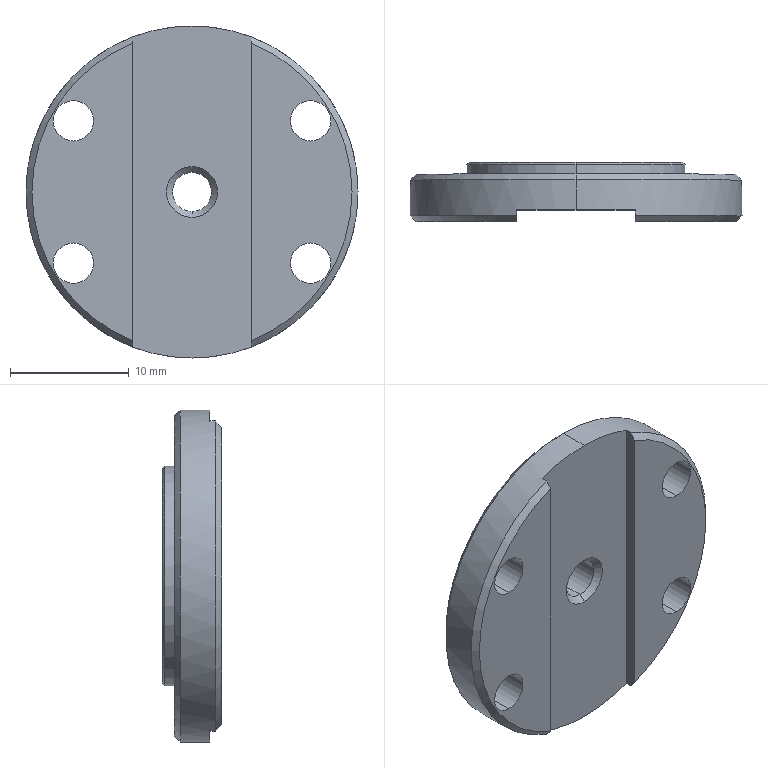Part | SolidWorks | features Chamfer 2, HoleWzd 2, ICE 2, Revolution 1 | 1 solid | 31 faces | box 28 x 5 x 28 mm | volume 2255 mm3 | cylinder 14 | cone 10 | plane 7 | commonest cylinder face diameters 3.4 x8 3.3 x2 18.5 x2 28 x2
STEP:
#1=CARTESIAN_POINT('',(0.,5.,9.05));
#2=VERTEX_POINT('',#1);
#3=CARTESIAN_POINT('',(0.,5.,-9.05));
#4=VERTEX_POINT('',#3);
#5=CARTESIAN_POINT('',(0.,5.,0.));
#6=DIRECTION('',(0.,1.,0.));
#7=DIRECTION('',(0.,0.,1.));
#8=AXIS2_PLACEMENT_3D('',#5,#6,#7);
#9=CIRCLE('',#8,9.05);
#10=EDGE_CURVE('',#2,#4,#9,.T.);
#11=ORIENTED_EDGE('',*,*,#10,.F.);
#12=CARTESIAN_POINT('',(0.,4.8,9.25));
#13=VERTEX_POINT('',#12);
#14=CARTESIAN_POINT('',(0.,5.,9.05));
#15=DIRECTION('',(0.,-0.7071,0.7071));
#16=VECTOR('',#15,1000.);
#17=LINE('',#14,#16);
#18=EDGE_CURVE('',#2,#13,#17,.T.);
#19=ORIENTED_EDGE('',*,*,#18,.T.);
#20=CARTESIAN_POINT('',(0.,4.8,-9.25));
#21=VERTEX_POINT('',#20);
#22=CARTESIAN_POINT('',(0.,4.8,0.));
#23=DIRECTION('',(0.,-1.,0.));
#24=DIRECTION('',(0.,0.,1.));
#25=AXIS2_PLACEMENT_3D('',#22,#23,#24);
#26=CIRCLE('',#25,9.25);
#27=EDGE_CURVE('',#21,#13,#26,.T.);
#28=ORIENTED_EDGE('',*,*,#27,.F.);
#29=CARTESIAN_POINT('',(0.,5.,-9.05));
#30=DIRECTION('',(0.,-0.7071,-0.7071));
#31=VECTOR('',#30,1000.);
#32=LINE('',#29,#31);
#33=EDGE_CURVE('',#4,#21,#32,.T.);
#34=ORIENTED_EDGE('',*,*,#33,.F.);
#35=EDGE_LOOP('',(#11,#19,#28,#34));
#36=FACE_OUTER_BOUND('',#35,.T.);
#37=CARTESIAN_POINT('',(0.,5.,0.));
#38=DIRECTION('',(0.,-1.,0.));
#39=DIRECTION('',(0.,0.,-1.));
#40=AXIS2_PLACEMENT_3D('',#37,#38,#39);
#41=CONICAL_SURFACE('',#40,9.05,0.7854);
#42=ADVANCED_FACE('',(#36),#41,.T.);
#43=CARTESIAN_POINT('',(0.,4.,13.5));
#44=VERTEX_POINT('',#43);
#45=CARTESIAN_POINT('',(0.,4.,-13.5));
#46=VERTEX_POINT('',#45);
#47=CARTESIAN_POINT('',(0.,4.,0.));
#48=DIRECTION('',(0.,1.,0.));
#49=DIRECTION('',(0.,0.,1.));
#50=AXIS2_PLACEMENT_3D('',#47,#48,#49);
#51=CIRCLE('',#50,13.5);
#52=EDGE_CURVE('',#44,#46,#51,.T.);
#53=ORIENTED_EDGE('',*,*,#52,.F.);
#54=CARTESIAN_POINT('',(0.,3.5,14.));
#55=VERTEX_POINT('',#54);
#56=CARTESIAN_POINT('',(0.,3.5,14.));
#57=DIRECTION('',(0.,-0.7071,0.7071));
#58=VECTOR('',#57,1000.);
#59=LINE('',#56,#58);
#60=EDGE_CURVE('',#44,#55,#59,.T.);
#61=ORIENTED_EDGE('',*,*,#60,.T.);
#62=CARTESIAN_POINT('',(0.,3.5,-14.));
#63=VERTEX_POINT('',#62);
#64=CARTESIAN_POINT('',(0.,3.5,0.));
#65=DIRECTION('',(0.,-1.,0.));
#66=DIRECTION('',(0.,0.,1.));
#67=AXIS2_PLACEMENT_3D('',#64,#65,#66);
#68=CIRCLE('',#67,14.);
#69=EDGE_CURVE('',#63,#55,#68,.T.);
#70=ORIENTED_EDGE('',*,*,#69,.F.);
#71=CARTESIAN_POINT('',(0.,3.5,-14.));
#72=DIRECTION('',(0.,-0.7071,-0.7071));
#73=VECTOR('',#72,1000.);
#74=LINE('',#71,#73);
#75=EDGE_CURVE('',#46,#63,#74,.T.);
#76=ORIENTED_EDGE('',*,*,#75,.F.);
#77=EDGE_LOOP('',(#53,#61,#70,#76));
#78=FACE_OUTER_BOUND('',#77,.T.);
#79=CARTESIAN_POINT('',(0.,3.5,0.));
#80=DIRECTION('',(0.,-1.,0.));
#81=DIRECTION('',(0.,0.,-1.));
#82=AXIS2_PLACEMENT_3D('',#79,#80,#81);
#83=CONICAL_SURFACE('',#82,14.,0.7854);
#84=ADVANCED_FACE('',(#78),#83,.T.);
#85=CARTESIAN_POINT('',(0.,4.5,-1.65));
#86=VERTEX_POINT('',#85);
#87=CARTESIAN_POINT('',(0.,4.5,1.65));
#88=VERTEX_POINT('',#87);
#89=CARTESIAN_POINT('',(0.,4.5,0.));
#90=DIRECTION('',(0.,1.,0.));
#91=DIRECTION('',(0.,0.,1.));
#92=AXIS2_PLACEMENT_3D('',#89,#90,#91);
#93=CIRCLE('',#92,1.65);
#94=EDGE_CURVE('',#86,#88,#93,.T.);
#95=ORIENTED_EDGE('',*,*,#94,.F.);
#96=CARTESIAN_POINT('',(0.,5.,-2.15));
#97=VERTEX_POINT('',#96);
#98=CARTESIAN_POINT('',(0.,4.5,-1.65));
#99=DIRECTION('',(0.,0.7071,-0.7071));
#100=VECTOR('',#99,1000.);
#101=LINE('',#98,#100);
#102=EDGE_CURVE('',#86,#97,#101,.T.);
#103=ORIENTED_EDGE('',*,*,#102,.T.);
#104=CARTESIAN_POINT('',(0.,5.,2.15));
#105=VERTEX_POINT('',#104);
#106=CARTESIAN_POINT('',(0.,5.,0.));
#107=DIRECTION('',(0.,-1.,0.));
#108=DIRECTION('',(0.,0.,1.));
#109=AXIS2_PLACEMENT_3D('',#106,#107,#108);
#110=CIRCLE('',#109,2.15);
#111=EDGE_CURVE('',#105,#97,#110,.T.);
#112=ORIENTED_EDGE('',*,*,#111,.F.);
#113=CARTESIAN_POINT('',(0.,4.5,1.65));
#114=DIRECTION('',(0.,0.7071,0.7071));
#115=VECTOR('',#114,1000.);
#116=LINE('',#113,#115);
#117=EDGE_CURVE('',#88,#105,#116,.T.);
#118=ORIENTED_EDGE('',*,*,#117,.F.);
#119=EDGE_LOOP('',(#95,#103,#112,#118));
#120=FACE_OUTER_BOUND('',#119,.T.);
#121=CARTESIAN_POINT('',(0.,4.5,0.));
#122=DIRECTION('',(0.,1.,0.));
#123=DIRECTION('',(0.,0.,1.));
#124=AXIS2_PLACEMENT_3D('',#121,#122,#123);
#125=CONICAL_SURFACE('',#124,1.65,0.7854);
#126=ADVANCED_FACE('',(#120),#125,.F.);
#127=CARTESIAN_POINT('',(0.,1.5,1.65));
#128=VERTEX_POINT('',#127);
#129=CARTESIAN_POINT('',(0.,1.5,-1.65));
#130=VERTEX_POINT('',#129);
#131=CARTESIAN_POINT('',(0.,1.5,0.));
#132=DIRECTION('',(0.,-1.,0.));
#133=DIRECTION('',(0.,0.,1.));
#134=AXIS2_PLACEMENT_3D('',#131,#132,#133);
#135=CIRCLE('',#134,1.65);
#136=EDGE_CURVE('',#128,#130,#135,.T.);
#137=ORIENTED_EDGE('',*,*,#136,.F.);
#138=CARTESIAN_POINT('',(0.,1.,2.15));
#139=VERTEX_POINT('',#138);
#140=CARTESIAN_POINT('',(0.,1.5,1.65));
#141=DIRECTION('',(0.,-0.7071,0.7071));
#142=VECTOR('',#141,1000.);
#143=LINE('',#140,#142);
#144=EDGE_CURVE('',#128,#139,#143,.T.);
#145=ORIENTED_EDGE('',*,*,#144,.T.);
#146=CARTESIAN_POINT('',(0.,1.,-2.15));
#147=VERTEX_POINT('',#146);
#148=CARTESIAN_POINT('',(0.,1.,0.));
#149=DIRECTION('',(0.,1.,0.));
#150=DIRECTION('',(0.,0.,1.));
#151=AXIS2_PLACEMENT_3D('',#148,#149,#150);
#152=CIRCLE('',#151,2.15);
#153=EDGE_CURVE('',#147,#139,#152,.T.);
#154=ORIENTED_EDGE('',*,*,#153,.F.);
#155=CARTESIAN_POINT('',(0.,1.5,-1.65));
#156=DIRECTION('',(0.,-0.7071,-0.7071));
#157=VECTOR('',#156,1000.);
#158=LINE('',#155,#157);
#159=EDGE_CURVE('',#130,#147,#158,.T.);
#160=ORIENTED_EDGE('',*,*,#159,.F.);
#161=EDGE_LOOP('',(#137,#145,#154,#160));
#162=FACE_OUTER_BOUND('',#161,.T.);
#163=CARTESIAN_POINT('',(0.,1.5,0.));
#164=DIRECTION('',(0.,-1.,0.));
#165=DIRECTION('',(0.,0.,-1.));
#166=AXIS2_PLACEMENT_3D('',#163,#164,#165);
#167=CONICAL_SURFACE('',#166,1.65,0.7854);
#168=ADVANCED_FACE('',(#162),#167,.F.);
#169=ORIENTED_EDGE('',*,*,#94,.T.);
#170=CARTESIAN_POINT('',(0.,1.,1.65));
#171=DIRECTION('',(0.,-1.,0.));
#172=VECTOR('',#171,1000.);
#173=LINE('',#170,#172);
#174=EDGE_CURVE('',#88,#128,#173,.T.);
#175=ORIENTED_EDGE('',*,*,#174,.T.);
#176=ORIENTED_EDGE('',*,*,#136,.T.);
#177=CARTESIAN_POINT('',(0.,1.,-1.65));
#178=DIRECTION('',(0.,-1.,0.));
#179=VECTOR('',#178,1000.);
#180=LINE('',#177,#179);
#181=EDGE_CURVE('',#86,#130,#180,.T.);
#182=ORIENTED_EDGE('',*,*,#181,.F.);
#183=EDGE_LOOP('',(#169,#175,#176,#182));
#184=FACE_OUTER_BOUND('',#183,.T.);
#185=CARTESIAN_POINT('',(0.,1.,0.));
#186=DIRECTION('',(0.,-1.,0.));
#187=DIRECTION('',(0.,0.,-1.));
#188=AXIS2_PLACEMENT_3D('',#185,#186,#187);
#189=CYLINDRICAL_SURFACE('',#188,1.65);
#190=ADVANCED_FACE('',(#184),#189,.F.);
#191=CARTESIAN_POINT('',(-10.,4.,4.3));
#192=VERTEX_POINT('',#191);
#193=CARTESIAN_POINT('',(-10.,4.,7.7));
#194=VERTEX_POINT('',#193);
#195=CARTESIAN_POINT('',(-10.,4.,6.));
#196=DIRECTION('',(0.,1.,0.));
#197=DIRECTION('',(0.,0.,1.));
#198=AXIS2_PLACEMENT_3D('',#195,#196,#197);
#199=CIRCLE('',#198,1.7);
#200=EDGE_CURVE('',#192,#194,#199,.T.);
#201=ORIENTED_EDGE('',*,*,#200,.T.);
#202=CARTESIAN_POINT('',(-10.,0.,7.7));
#203=VERTEX_POINT('',#202);
#204=CARTESIAN_POINT('',(-10.,0.,7.7));
#205=DIRECTION('',(0.,-1.,0.));
#206=VECTOR('',#205,1000.);
#207=LINE('',#204,#206);
#208=EDGE_CURVE('',#194,#203,#207,.T.);
#209=ORIENTED_EDGE('',*,*,#208,.T.);
#210=CARTESIAN_POINT('',(-10.,0.,4.3));
#211=VERTEX_POINT('',#210);
#212=CARTESIAN_POINT('',(-10.,0.,6.));
#213=DIRECTION('',(0.,-1.,0.));
#214=DIRECTION('',(0.,0.,-1.));
#215=AXIS2_PLACEMENT_3D('',#212,#213,#214);
#216=CIRCLE('',#215,1.7);
#217=EDGE_CURVE('',#203,#211,#216,.T.);
#218=ORIENTED_EDGE('',*,*,#217,.T.);
#219=CARTESIAN_POINT('',(-10.,0.,4.3));
#220=DIRECTION('',(0.,-1.,0.));
#221=VECTOR('',#220,1000.);
#222=LINE('',#219,#221);
#223=EDGE_CURVE('',#192,#211,#222,.T.);
#224=ORIENTED_EDGE('',*,*,#223,.F.);
#225=EDGE_LOOP('',(#201,#209,#218,#224));
#226=FACE_OUTER_BOUND('',#225,.T.);
#227=CARTESIAN_POINT('',(-10.,0.,6.));
#228=DIRECTION('',(0.,-1.,0.));
#229=DIRECTION('',(0.,0.,-1.));
#230=AXIS2_PLACEMENT_3D('',#227,#228,#229);
#231=CYLINDRICAL_SURFACE('',#230,1.7);
#232=ADVANCED_FACE('',(#226),#231,.F.);
#233=CARTESIAN_POINT('',(-10.,4.,-7.7));
#234=VERTEX_POINT('',#233);
#235=CARTESIAN_POINT('',(-10.,4.,-4.3));
#236=VERTEX_POINT('',#235);
#237=CARTESIAN_POINT('',(-10.,4.,-6.));
#238=DIRECTION('',(0.,1.,0.));
#239=DIRECTION('',(0.,0.,1.));
#240=AXIS2_PLACEMENT_3D('',#237,#238,#239);
#241=CIRCLE('',#240,1.7);
#242=EDGE_CURVE('',#234,#236,#241,.T.);
#243=ORIENTED_EDGE('',*,*,#242,.T.);
#244=CARTESIAN_POINT('',(-10.,0.,-4.3));
#245=VERTEX_POINT('',#244);
#246=CARTESIAN_POINT('',(-10.,0.,-4.3));
#247=DIRECTION('',(0.,-1.,0.));
#248=VECTOR('',#247,1000.);
#249=LINE('',#246,#248);
#250=EDGE_CURVE('',#236,#245,#249,.T.);
#251=ORIENTED_EDGE('',*,*,#250,.T.);
#252=CARTESIAN_POINT('',(-10.,0.,-7.7));
#253=VERTEX_POINT('',#252);
#254=CARTESIAN_POINT('',(-10.,0.,-6.));
#255=DIRECTION('',(0.,-1.,0.));
#256=DIRECTION('',(0.,0.,-1.));
#257=AXIS2_PLACEMENT_3D('',#254,#255,#256);
#258=CIRCLE('',#257,1.7);
#259=EDGE_CURVE('',#245,#253,#258,.T.);
#260=ORIENTED_EDGE('',*,*,#259,.T.);
#261=CARTESIAN_POINT('',(-10.,0.,-7.7));
#262=DIRECTION('',(0.,-1.,0.));
#263=VECTOR('',#262,1000.);
#264=LINE('',#261,#263);
#265=EDGE_CURVE('',#234,#253,#264,.T.);
#266=ORIENTED_EDGE('',*,*,#265,.F.);
#267=EDGE_LOOP('',(#243,#251,#260,#266));
#268=FACE_OUTER_BOUND('',#267,.T.);
#269=CARTESIAN_POINT('',(-10.,0.,-6.));
#270=DIRECTION('',(0.,-1.,0.));
#271=DIRECTION('',(0.,0.,-1.));
#272=AXIS2_PLACEMENT_3D('',#269,#270,#271);
#273=CYLINDRICAL_SURFACE('',#272,1.7);
#274=ADVANCED_FACE('',(#268),#273,.F.);
#275=CARTESIAN_POINT('',(10.,4.,4.3));
#276=VERTEX_POINT('',#275);
#277=CARTESIAN_POINT('',(10.,4.,7.7));
#278=VERTEX_POINT('',#277);
#279=CARTESIAN_POINT('',(10.,4.,6.));
#280=DIRECTION('',(0.,1.,0.));
#281=DIRECTION('',(0.,0.,1.));
#282=AXIS2_PLACEMENT_3D('',#279,#280,#281);
#283=CIRCLE('',#282,1.7);
#284=EDGE_CURVE('',#276,#278,#283,.T.);
#285=ORIENTED_EDGE('',*,*,#284,.T.);
#286=CARTESIAN_POINT('',(10.,0.,7.7));
#287=VERTEX_POINT('',#286);
#288=CARTESIAN_POINT('',(10.,0.,7.7));
#289=DIRECTION('',(0.,-1.,0.));
#290=VECTOR('',#289,1000.);
#291=LINE('',#288,#290);
#292=EDGE_CURVE('',#278,#287,#291,.T.);
#293=ORIENTED_EDGE('',*,*,#292,.T.);
#294=CARTESIAN_POINT('',(10.,0.,4.3));
#295=VERTEX_POINT('',#294);
#296=CARTESIAN_POINT('',(10.,0.,6.));
#297=DIRECTION('',(0.,-1.,0.));
#298=DIRECTION('',(0.,0.,-1.));
#299=AXIS2_PLACEMENT_3D('',#296,#297,#298);
#300=CIRCLE('',#299,1.7);
#301=EDGE_CURVE('',#287,#295,#300,.T.);
#302=ORIENTED_EDGE('',*,*,#301,.T.);
#303=CARTESIAN_POINT('',(10.,0.,4.3));
#304=DIRECTION('',(0.,-1.,0.));
#305=VECTOR('',#304,1000.);
#306=LINE('',#303,#305);
#307=EDGE_CURVE('',#276,#295,#306,.T.);
#308=ORIENTED_EDGE('',*,*,#307,.F.);
#309=EDGE_LOOP('',(#285,#293,#302,#308));
#310=FACE_OUTER_BOUND('',#309,.T.);
#311=CARTESIAN_POINT('',(10.,0.,6.));
#312=DIRECTION('',(0.,-1.,0.));
#313=DIRECTION('',(0.,0.,-1.));
#314=AXIS2_PLACEMENT_3D('',#311,#312,#313);
#315=CYLINDRICAL_SURFACE('',#314,1.7);
#316=ADVANCED_FACE('',(#310),#315,.F.);
#317=CARTESIAN_POINT('',(10.,4.,-7.7));
#318=VERTEX_POINT('',#317);
#319=CARTESIAN_POINT('',(10.,4.,-4.3));
#320=VERTEX_POINT('',#319);
#321=CARTESIAN_POINT('',(10.,4.,-6.));
#322=DIRECTION('',(0.,1.,0.));
#323=DIRECTION('',(0.,0.,1.));
#324=AXIS2_PLACEMENT_3D('',#321,#322,#323);
#325=CIRCLE('',#324,1.7);
#326=EDGE_CURVE('',#318,#320,#325,.T.);
#327=ORIENTED_EDGE('',*,*,#326,.T.);
#328=CARTESIAN_POINT('',(10.,0.,-4.3));
#329=VERTEX_POINT('',#328);
#330=CARTESIAN_POINT('',(10.,0.,-4.3));
#331=DIRECTION('',(0.,-1.,0.));
#332=VECTOR('',#331,1000.);
#333=LINE('',#330,#332);
#334=EDGE_CURVE('',#320,#329,#333,.T.);
#335=ORIENTED_EDGE('',*,*,#334,.T.);
#336=CARTESIAN_POINT('',(10.,0.,-7.7));
#337=VERTEX_POINT('',#336);
#338=CARTESIAN_POINT('',(10.,0.,-6.));
#339=DIRECTION('',(0.,-1.,0.));
#340=DIRECTION('',(0.,0.,-1.));
#341=AXIS2_PLACEMENT_3D('',#338,#339,#340);
#342=CIRCLE('',#341,1.7);
#343=EDGE_CURVE('',#329,#337,#342,.T.);
#344=ORIENTED_EDGE('',*,*,#343,.T.);
#345=CARTESIAN_POINT('',(10.,0.,-7.7));
#346=DIRECTION('',(0.,-1.,0.));
#347=VECTOR('',#346,1000.);
#348=LINE('',#345,#347);
#349=EDGE_CURVE('',#318,#337,#348,.T.);
#350=ORIENTED_EDGE('',*,*,#349,.F.);
#351=EDGE_LOOP('',(#327,#335,#344,#350));
#352=FACE_OUTER_BOUND('',#351,.T.);
#353=CARTESIAN_POINT('',(10.,0.,-6.));
#354=DIRECTION('',(0.,-1.,0.));
#355=DIRECTION('',(0.,0.,-1.));
#356=AXIS2_PLACEMENT_3D('',#353,#354,#355);
#357=CYLINDRICAL_SURFACE('',#356,1.7);
#358=ADVANCED_FACE('',(#352),#357,.F.);
#359=CARTESIAN_POINT('',(0.,4.,9.25));
#360=VERTEX_POINT('',#359);
#361=CARTESIAN_POINT('',(0.,4.,-9.25));
#362=VERTEX_POINT('',#361);
#363=CARTESIAN_POINT('',(0.,4.,0.));
#364=DIRECTION('',(0.,1.,0.));
#365=DIRECTION('',(0.,0.,1.));
#366=AXIS2_PLACEMENT_3D('',#363,#364,#365);
#367=CIRCLE('',#366,9.25);
#368=EDGE_CURVE('',#360,#362,#367,.T.);
#369=ORIENTED_EDGE('',*,*,#368,.T.);
#370=CARTESIAN_POINT('',(0.,4.,-9.25));
#371=DIRECTION('',(0.,1.,0.));
#372=VECTOR('',#371,1000.);
#373=LINE('',#370,#372);
#374=EDGE_CURVE('',#362,#21,#373,.T.);
#375=ORIENTED_EDGE('',*,*,#374,.T.);
#376=ORIENTED_EDGE('',*,*,#27,.T.);
#377=CARTESIAN_POINT('',(0.,4.,9.25));
#378=DIRECTION('',(0.,1.,0.));
#379=VECTOR('',#378,1000.);
#380=LINE('',#377,#379);
#381=EDGE_CURVE('',#360,#13,#380,.T.);
#382=ORIENTED_EDGE('',*,*,#381,.F.);
#383=EDGE_LOOP('',(#369,#375,#376,#382));
#384=FACE_OUTER_BOUND('',#383,.T.);
#385=CARTESIAN_POINT('',(0.,4.,0.));
#386=DIRECTION('',(0.,1.,0.));
#387=DIRECTION('',(0.,0.,1.));
#388=AXIS2_PLACEMENT_3D('',#385,#386,#387);
#389=CYLINDRICAL_SURFACE('',#388,9.25);
#390=ADVANCED_FACE('',(#384),#389,.T.);
#391=ORIENTED_EDGE('',*,*,#69,.T.);
#392=CARTESIAN_POINT('',(0.,1.,14.));
#393=VERTEX_POINT('',#392);
#394=CARTESIAN_POINT('',(0.,0.,14.));
#395=DIRECTION('',(0.,-1.,0.));
#396=VECTOR('',#395,1000.);
#397=LINE('',#394,#396);
#398=EDGE_CURVE('',#55,#393,#397,.T.);
#399=ORIENTED_EDGE('',*,*,#398,.T.);
#400=CARTESIAN_POINT('',(5.,1.,13.077));
#401=VERTEX_POINT('',#400);
#402=CARTESIAN_POINT('',(0.,1.,0.));
#403=DIRECTION('',(0.,-1.,0.));
#404=DIRECTION('',(0.,0.,1.));
#405=AXIS2_PLACEMENT_3D('',#402,#403,#404);
#406=CIRCLE('',#405,14.);
#407=EDGE_CURVE('',#401,#393,#406,.T.);
#408=ORIENTED_EDGE('',*,*,#407,.F.);
#409=CARTESIAN_POINT('',(5.,0.5,13.077));
#410=VERTEX_POINT('',#409);
#411=CARTESIAN_POINT('',(5.,0.,13.077));
#412=DIRECTION('',(0.,1.,0.));
#413=VECTOR('',#412,1000.);
#414=LINE('',#411,#413);
#415=EDGE_CURVE('',#410,#401,#414,.T.);
#416=ORIENTED_EDGE('',*,*,#415,.F.);
#417=CARTESIAN_POINT('',(5.,0.5,-13.077));
#418=VERTEX_POINT('',#417);
#419=CARTESIAN_POINT('',(0.,0.5,0.));
#420=DIRECTION('',(0.,1.,0.));
#421=DIRECTION('',(0.,0.,-1.));
#422=AXIS2_PLACEMENT_3D('',#419,#420,#421);
#423=CIRCLE('',#422,14.);
#424=EDGE_CURVE('',#410,#418,#423,.T.);
#425=ORIENTED_EDGE('',*,*,#424,.T.);
#426=CARTESIAN_POINT('',(5.,1.,-13.077));
#427=VERTEX_POINT('',#426);
#428=CARTESIAN_POINT('',(5.,0.,-13.077));
#429=DIRECTION('',(0.,-1.,0.));
#430=VECTOR('',#429,1000.);
#431=LINE('',#428,#430);
#432=EDGE_CURVE('',#427,#418,#431,.T.);
#433=ORIENTED_EDGE('',*,*,#432,.F.);
#434=CARTESIAN_POINT('',(0.,1.,-14.));
#435=VERTEX_POINT('',#434);
#436=CARTESIAN_POINT('',(0.,1.,0.));
#437=DIRECTION('',(0.,-1.,0.));
#438=DIRECTION('',(0.,0.,1.));
#439=AXIS2_PLACEMENT_3D('',#436,#437,#438);
#440=CIRCLE('',#439,14.);
#441=EDGE_CURVE('',#435,#427,#440,.T.);
#442=ORIENTED_EDGE('',*,*,#441,.F.);
#443=CARTESIAN_POINT('',(0.,0.,-14.));
#444=DIRECTION('',(0.,-1.,0.));
#445=VECTOR('',#444,1000.);
#446=LINE('',#443,#445);
#447=EDGE_CURVE('',#63,#435,#446,.T.);
#448=ORIENTED_EDGE('',*,*,#447,.F.);
#449=EDGE_LOOP('',(#391,#399,#408,#416,#425,#433,#442,#448));
#450=FACE_OUTER_BOUND('',#449,.T.);
#451=CARTESIAN_POINT('',(0.,0.,0.));
#452=DIRECTION('',(0.,-1.,0.));
#453=DIRECTION('',(0.,0.,-1.));
#454=AXIS2_PLACEMENT_3D('',#451,#452,#453);
#455=CYLINDRICAL_SURFACE('',#454,14.);
#456=ADVANCED_FACE('',(#450),#455,.T.);
#457=CARTESIAN_POINT('',(-5.,0.,12.54));
#458=VERTEX_POINT('',#457);
#459=CARTESIAN_POINT('',(-5.,0.,-12.54));
#460=VERTEX_POINT('',#459);
#461=CARTESIAN_POINT('',(-5.,0.,0.));
#462=DIRECTION('',(0.,0.,-1.));
#463=VECTOR('',#462,1000.);
#464=LINE('',#461,#463);
#465=EDGE_CURVE('',#458,#460,#464,.T.);
#466=ORIENTED_EDGE('',*,*,#465,.F.);
#467=CARTESIAN_POINT('',(0.,0.,0.));
#468=DIRECTION('',(0.,-1.,0.));
#469=DIRECTION('',(0.,0.,-1.));
#470=AXIS2_PLACEMENT_3D('',#467,#468,#469);
#471=CIRCLE('',#470,13.5);
#472=EDGE_CURVE('',#458,#460,#471,.T.);
#473=ORIENTED_EDGE('',*,*,#472,.T.);
#474=EDGE_LOOP('',(#466,#473));
#475=FACE_OUTER_BOUND('',#474,.T.);
#476=CARTESIAN_POINT('',(-10.,0.,-6.));
#477=DIRECTION('',(0.,-1.,0.));
#478=DIRECTION('',(0.,0.,-1.));
#479=AXIS2_PLACEMENT_3D('',#476,#477,#478);
#480=CIRCLE('',#479,1.7);
#481=EDGE_CURVE('',#253,#245,#480,.T.);
#482=ORIENTED_EDGE('',*,*,#481,.F.);
#483=ORIENTED_EDGE('',*,*,#259,.F.);
#484=EDGE_LOOP('',(#482,#483));
#485=FACE_BOUND('',#484,.T.);
#486=CARTESIAN_POINT('',(-10.,0.,6.));
#487=DIRECTION('',(0.,-1.,0.));
#488=DIRECTION('',(0.,0.,-1.));
#489=AXIS2_PLACEMENT_3D('',#486,#487,#488);
#490=CIRCLE('',#489,1.7);
#491=EDGE_CURVE('',#211,#203,#490,.T.);
#492=ORIENTED_EDGE('',*,*,#491,.F.);
#493=ORIENTED_EDGE('',*,*,#217,.F.);
#494=EDGE_LOOP('',(#492,#493));
#495=FACE_BOUND('',#494,.T.);
#496=CARTESIAN_POINT('',(0.,0.,0.));
#497=DIRECTION('',(0.,-1.,0.));
#498=DIRECTION('',(0.,0.,-1.));
#499=AXIS2_PLACEMENT_3D('',#496,#497,#498);
#500=PLANE('',#499);
#501=ADVANCED_FACE('',(#475,#485,#495),#500,.T.);
#502=ORIENTED_EDGE('',*,*,#398,.F.);
#503=CARTESIAN_POINT('',(0.,3.5,0.));
#504=DIRECTION('',(0.,-1.,0.));
#505=DIRECTION('',(0.,0.,1.));
#506=AXIS2_PLACEMENT_3D('',#503,#504,#505);
#507=CIRCLE('',#506,14.);
#508=EDGE_CURVE('',#55,#63,#507,.T.);
#509=ORIENTED_EDGE('',*,*,#508,.T.);
#510=ORIENTED_EDGE('',*,*,#447,.T.);
#511=CARTESIAN_POINT('',(-5.,1.,-13.077));
#512=VERTEX_POINT('',#511);
#513=CARTESIAN_POINT('',(0.,1.,0.));
#514=DIRECTION('',(0.,-1.,0.));
#515=DIRECTION('',(0.,0.,1.));
#516=AXIS2_PLACEMENT_3D('',#513,#514,#515);
#517=CIRCLE('',#516,14.);
#518=EDGE_CURVE('',#512,#435,#517,.T.);
#519=ORIENTED_EDGE('',*,*,#518,.F.);
#520=CARTESIAN_POINT('',(-5.,0.5,-13.077));
#521=VERTEX_POINT('',#520);
#522=CARTESIAN_POINT('',(-5.,0.,-13.077));
#523=DIRECTION('',(0.,1.,0.));
#524=VECTOR('',#523,1000.);
#525=LINE('',#522,#524);
#526=EDGE_CURVE('',#521,#512,#525,.T.);
#527=ORIENTED_EDGE('',*,*,#526,.F.);
#528=CARTESIAN_POINT('',(-5.,0.5,13.077));
#529=VERTEX_POINT('',#528);
#530=CARTESIAN_POINT('',(0.,0.5,0.));
#531=DIRECTION('',(0.,1.,0.));
#532=DIRECTION('',(0.,0.,-1.));
#533=AXIS2_PLACEMENT_3D('',#530,#531,#532);
#534=CIRCLE('',#533,14.);
#535=EDGE_CURVE('',#521,#529,#534,.T.);
#536=ORIENTED_EDGE('',*,*,#535,.T.);
#537=CARTESIAN_POINT('',(-5.,1.,13.077));
#538=VERTEX_POINT('',#537);
#539=CARTESIAN_POINT('',(-5.,0.,13.077));
#540=DIRECTION('',(0.,-1.,0.));
#541=VECTOR('',#540,1000.);
#542=LINE('',#539,#541);
#543=EDGE_CURVE('',#538,#529,#542,.T.);
#544=ORIENTED_EDGE('',*,*,#543,.F.);
#545=CARTESIAN_POINT('',(0.,1.,0.));
#546=DIRECTION('',(0.,-1.,0.));
#547=DIRECTION('',(0.,0.,1.));
#548=AXIS2_PLACEMENT_3D('',#545,#546,#547);
#549=CIRCLE('',#548,14.);
#550=EDGE_CURVE('',#393,#538,#549,.T.);
#551=ORIENTED_EDGE('',*,*,#550,.F.);
#552=EDGE_LOOP('',(#502,#509,#510,#519,#527,#536,#544,#551));
#553=FACE_OUTER_BOUND('',#552,.T.);
#554=CARTESIAN_POINT('',(0.,0.,0.));
#555=DIRECTION('',(0.,-1.,0.));
#556=DIRECTION('',(0.,0.,-1.));
#557=AXIS2_PLACEMENT_3D('',#554,#555,#556);
#558=CYLINDRICAL_SURFACE('',#557,14.);
#559=ADVANCED_FACE('',(#553),#558,.T.);
#560=CARTESIAN_POINT('',(5.,0.,-12.54));
#561=VERTEX_POINT('',#560);
#562=CARTESIAN_POINT('',(5.,0.,12.54));
#563=VERTEX_POINT('',#562);
#564=CARTESIAN_POINT('',(5.,0.,0.));
#565=DIRECTION('',(0.,0.,1.));
#566=VECTOR('',#565,1000.);
#567=LINE('',#564,#566);
#568=EDGE_CURVE('',#561,#563,#567,.T.);
#569=ORIENTED_EDGE('',*,*,#568,.F.);
#570=CARTESIAN_POINT('',(0.,0.,0.));
#571=DIRECTION('',(0.,-1.,0.));
#572=DIRECTION('',(0.,0.,-1.));
#573=AXIS2_PLACEMENT_3D('',#570,#571,#572);
#574=CIRCLE('',#573,13.5);
#575=EDGE_CURVE('',#561,#563,#574,.T.);
#576=ORIENTED_EDGE('',*,*,#575,.T.);
#577=EDGE_LOOP('',(#569,#576));
#578=FACE_OUTER_BOUND('',#577,.T.);
#579=CARTESIAN_POINT('',(10.,0.,6.));
#580=DIRECTION('',(0.,-1.,0.));
#581=DIRECTION('',(0.,0.,-1.));
#582=AXIS2_PLACEMENT_3D('',#579,#580,#581);
#583=CIRCLE('',#582,1.7);
#584=EDGE_CURVE('',#295,#287,#583,.T.);
#585=ORIENTED_EDGE('',*,*,#584,.F.);
#586=ORIENTED_EDGE('',*,*,#301,.F.);
#587=EDGE_LOOP('',(#585,#586));
#588=FACE_BOUND('',#587,.T.);
#589=CARTESIAN_POINT('',(10.,0.,-6.));
#590=DIRECTION('',(0.,-1.,0.));
#591=DIRECTION('',(0.,0.,-1.));
#592=AXIS2_PLACEMENT_3D('',#589,#590,#591);
#593=CIRCLE('',#592,1.7);
#594=EDGE_CURVE('',#337,#329,#593,.T.);
#595=ORIENTED_EDGE('',*,*,#594,.F.);
#596=ORIENTED_EDGE('',*,*,#343,.F.);
#597=EDGE_LOOP('',(#595,#596));
#598=FACE_BOUND('',#597,.T.);
#599=CARTESIAN_POINT('',(0.,0.,0.));
#600=DIRECTION('',(0.,-1.,0.));
#601=DIRECTION('',(0.,0.,-1.));
#602=AXIS2_PLACEMENT_3D('',#599,#600,#601);
#603=PLANE('',#602);
#604=ADVANCED_FACE('',(#578,#588,#598),#603,.T.);
#605=CARTESIAN_POINT('',(0.,4.,0.));
#606=DIRECTION('',(0.,1.,0.));
#607=DIRECTION('',(0.,0.,1.));
#608=AXIS2_PLACEMENT_3D('',#605,#606,#607);
#609=CIRCLE('',#608,13.5);
#610=EDGE_CURVE('',#46,#44,#609,.T.);
#611=ORIENTED_EDGE('',*,*,#610,.T.);
#612=ORIENTED_EDGE('',*,*,#52,.T.);
#613=EDGE_LOOP('',(#611,#612));
#614=FACE_OUTER_BOUND('',#613,.T.);
#615=ORIENTED_EDGE('',*,*,#200,.F.);
#616=CARTESIAN_POINT('',(-10.,4.,6.));
#617=DIRECTION('',(0.,1.,0.));
#618=DIRECTION('',(0.,0.,1.));
#619=AXIS2_PLACEMENT_3D('',#616,#617,#618);
#620=CIRCLE('',#619,1.7);
#621=EDGE_CURVE('',#194,#192,#620,.T.);
#622=ORIENTED_EDGE('',*,*,#621,.F.);
#623=EDGE_LOOP('',(#615,#622));
#624=FACE_BOUND('',#623,.T.);
#625=ORIENTED_EDGE('',*,*,#242,.F.);
#626=CARTESIAN_POINT('',(-10.,4.,-6.));
#627=DIRECTION('',(0.,1.,0.));
#628=DIRECTION('',(0.,0.,1.));
#629=AXIS2_PLACEMENT_3D('',#626,#627,#628);
#630=CIRCLE('',#629,1.7);
#631=EDGE_CURVE('',#236,#234,#630,.T.);
#632=ORIENTED_EDGE('',*,*,#631,.F.);
#633=EDGE_LOOP('',(#625,#632));
#634=FACE_BOUND('',#633,.T.);
#635=ORIENTED_EDGE('',*,*,#284,.F.);
#636=CARTESIAN_POINT('',(10.,4.,6.));
#637=DIRECTION('',(0.,1.,0.));
#638=DIRECTION('',(0.,0.,1.));
#639=AXIS2_PLACEMENT_3D('',#636,#637,#638);
#640=CIRCLE('',#639,1.7);
#641=EDGE_CURVE('',#278,#276,#640,.T.);
#642=ORIENTED_EDGE('',*,*,#641,.F.);
#643=EDGE_LOOP('',(#635,#642));
#644=FACE_BOUND('',#643,.T.);
#645=ORIENTED_EDGE('',*,*,#326,.F.);
#646=CARTESIAN_POINT('',(10.,4.,-6.));
#647=DIRECTION('',(0.,1.,0.));
#648=DIRECTION('',(0.,0.,1.));
#649=AXIS2_PLACEMENT_3D('',#646,#647,#648);
#650=CIRCLE('',#649,1.7);
#651=EDGE_CURVE('',#320,#318,#650,.T.);
#652=ORIENTED_EDGE('',*,*,#651,.F.);
#653=EDGE_LOOP('',(#645,#652));
#654=FACE_BOUND('',#653,.T.);
#655=ORIENTED_EDGE('',*,*,#368,.F.);
#656=CARTESIAN_POINT('',(0.,4.,0.));
#657=DIRECTION('',(0.,1.,0.));
#658=DIRECTION('',(0.,0.,1.));
#659=AXIS2_PLACEMENT_3D('',#656,#657,#658);
#660=CIRCLE('',#659,9.25);
#661=EDGE_CURVE('',#362,#360,#660,.T.);
#662=ORIENTED_EDGE('',*,*,#661,.F.);
#663=EDGE_LOOP('',(#655,#662));
#664=FACE_BOUND('',#663,.T.);
#665=CARTESIAN_POINT('',(0.,4.,0.));
#666=DIRECTION('',(0.,1.,0.));
#667=DIRECTION('',(0.,0.,1.));
#668=AXIS2_PLACEMENT_3D('',#665,#666,#667);
#669=PLANE('',#668);
#670=ADVANCED_FACE('',(#614,#624,#634,#644,#654,#664),#669,.T.);
#671=ORIENTED_EDGE('',*,*,#374,.F.);
#672=ORIENTED_EDGE('',*,*,#661,.T.);
#673=ORIENTED_EDGE('',*,*,#381,.T.);
#674=CARTESIAN_POINT('',(0.,4.8,0.));
#675=DIRECTION('',(0.,-1.,0.));
#676=DIRECTION('',(0.,0.,1.));
#677=AXIS2_PLACEMENT_3D('',#674,#675,#676);
#678=CIRCLE('',#677,9.25);
#679=EDGE_CURVE('',#13,#21,#678,.T.);
#680=ORIENTED_EDGE('',*,*,#679,.T.);
#681=EDGE_LOOP('',(#671,#672,#673,#680));
#682=FACE_OUTER_BOUND('',#681,.T.);
#683=CARTESIAN_POINT('',(0.,4.,0.));
#684=DIRECTION('',(0.,1.,0.));
#685=DIRECTION('',(0.,0.,1.));
#686=AXIS2_PLACEMENT_3D('',#683,#684,#685);
#687=CYLINDRICAL_SURFACE('',#686,9.25);
#688=ADVANCED_FACE('',(#682),#687,.T.);
#689=CARTESIAN_POINT('',(0.,5.,0.));
#690=DIRECTION('',(0.,1.,0.));
#691=DIRECTION('',(0.,0.,1.));
#692=AXIS2_PLACEMENT_3D('',#689,#690,#691);
#693=CIRCLE('',#692,9.05);
#694=EDGE_CURVE('',#4,#2,#693,.T.);
#695=ORIENTED_EDGE('',*,*,#694,.T.);
#696=ORIENTED_EDGE('',*,*,#10,.T.);
#697=EDGE_LOOP('',(#695,#696));
#698=FACE_OUTER_BOUND('',#697,.T.);
#699=ORIENTED_EDGE('',*,*,#111,.T.);
#700=CARTESIAN_POINT('',(0.,5.,0.));
#701=DIRECTION('',(0.,-1.,0.));
#702=DIRECTION('',(0.,0.,1.));
#703=AXIS2_PLACEMENT_3D('',#700,#701,#702);
#704=CIRCLE('',#703,2.15);
#705=EDGE_CURVE('',#97,#105,#704,.T.);
#706=ORIENTED_EDGE('',*,*,#705,.T.);
#707=EDGE_LOOP('',(#699,#706));
#708=FACE_BOUND('',#707,.T.);
#709=CARTESIAN_POINT('',(14.,5.,0.));
#710=DIRECTION('',(0.,1.,0.));
#711=DIRECTION('',(0.,0.,1.));
#712=AXIS2_PLACEMENT_3D('',#709,#710,#711);
#713=PLANE('',#712);
#714=ADVANCED_FACE('',(#698,#708),#713,.T.);
#715=ORIENTED_EDGE('',*,*,#334,.F.);
#716=ORIENTED_EDGE('',*,*,#651,.T.);
#717=ORIENTED_EDGE('',*,*,#349,.T.);
#718=ORIENTED_EDGE('',*,*,#594,.T.);
#719=EDGE_LOOP('',(#715,#716,#717,#718));
#720=FACE_OUTER_BOUND('',#719,.T.);
#721=CARTESIAN_POINT('',(10.,0.,-6.));
#722=DIRECTION('',(0.,-1.,0.));
#723=DIRECTION('',(0.,0.,-1.));
#724=AXIS2_PLACEMENT_3D('',#721,#722,#723);
#725=CYLINDRICAL_SURFACE('',#724,1.7);
#726=ADVANCED_FACE('',(#720),#725,.F.);
#727=ORIENTED_EDGE('',*,*,#292,.F.);
#728=ORIENTED_EDGE('',*,*,#641,.T.);
#729=ORIENTED_EDGE('',*,*,#307,.T.);
#730=ORIENTED_EDGE('',*,*,#584,.T.);
#731=EDGE_LOOP('',(#727,#728,#729,#730));
#732=FACE_OUTER_BOUND('',#731,.T.);
#733=CARTESIAN_POINT('',(10.,0.,6.));
#734=DIRECTION('',(0.,-1.,0.));
#735=DIRECTION('',(0.,0.,-1.));
#736=AXIS2_PLACEMENT_3D('',#733,#734,#735);
#737=CYLINDRICAL_SURFACE('',#736,1.7);
#738=ADVANCED_FACE('',(#732),#737,.F.);
#739=ORIENTED_EDGE('',*,*,#250,.F.);
#740=ORIENTED_EDGE('',*,*,#631,.T.);
#741=ORIENTED_EDGE('',*,*,#265,.T.);
#742=ORIENTED_EDGE('',*,*,#481,.T.);
#743=EDGE_LOOP('',(#739,#740,#741,#742));
#744=FACE_OUTER_BOUND('',#743,.T.);
#745=CARTESIAN_POINT('',(-10.,0.,-6.));
#746=DIRECTION('',(0.,-1.,0.));
#747=DIRECTION('',(0.,0.,-1.));
#748=AXIS2_PLACEMENT_3D('',#745,#746,#747);
#749=CYLINDRICAL_SURFACE('',#748,1.7);
#750=ADVANCED_FACE('',(#744),#749,.F.);
#751=ORIENTED_EDGE('',*,*,#208,.F.);
#752=ORIENTED_EDGE('',*,*,#621,.T.);
#753=ORIENTED_EDGE('',*,*,#223,.T.);
#754=ORIENTED_EDGE('',*,*,#491,.T.);
#755=EDGE_LOOP('',(#751,#752,#753,#754));
#756=FACE_OUTER_BOUND('',#755,.T.);
#757=CARTESIAN_POINT('',(-10.,0.,6.));
#758=DIRECTION('',(0.,-1.,0.));
#759=DIRECTION('',(0.,0.,-1.));
#760=AXIS2_PLACEMENT_3D('',#757,#758,#759);
#761=CYLINDRICAL_SURFACE('',#760,1.7);
#762=ADVANCED_FACE('',(#756),#761,.F.);
#763=ORIENTED_EDGE('',*,*,#465,.T.);
#764=CARTESIAN_POINT('',(-5.,0.,-12.54));
#765=CARTESIAN_POINT('',(-5.,0.1664,-12.719));
#766=CARTESIAN_POINT('',(-5.,0.3331,-12.898));
#767=CARTESIAN_POINT('',(-5.,0.5,-13.077));
#768=B_SPLINE_CURVE_WITH_KNOTS('',3,(#764,#765,#766,#767),.UNSPECIFIED.,.F.,.F.,(4,4),(0.,0.0007336),.UNSPECIFIED.);
#769=EDGE_CURVE('',#460,#521,#768,.T.);
#770=ORIENTED_EDGE('',*,*,#769,.T.);
#771=ORIENTED_EDGE('',*,*,#526,.T.);
#772=CARTESIAN_POINT('',(-5.,1.,15.714));
#773=DIRECTION('',(0.,0.,-1.));
#774=VECTOR('',#773,1000.);
#775=LINE('',#772,#774);
#776=EDGE_CURVE('',#538,#512,#775,.T.);
#777=ORIENTED_EDGE('',*,*,#776,.F.);
#778=ORIENTED_EDGE('',*,*,#543,.T.);
#779=CARTESIAN_POINT('',(-5.,0.5,13.077));
#780=CARTESIAN_POINT('',(-5.,0.3331,12.898));
#781=CARTESIAN_POINT('',(-5.,0.1664,12.719));
#782=CARTESIAN_POINT('',(-5.,0.,12.54));
#783=B_SPLINE_CURVE_WITH_KNOTS('',3,(#779,#780,#781,#782),.UNSPECIFIED.,.F.,.F.,(4,4),(0.,0.0007336),.UNSPECIFIED.);
#784=EDGE_CURVE('',#529,#458,#783,.T.);
#785=ORIENTED_EDGE('',*,*,#784,.T.);
#786=EDGE_LOOP('',(#763,#770,#771,#777,#778,#785));
#787=FACE_OUTER_BOUND('',#786,.T.);
#788=CARTESIAN_POINT('',(-5.,1.,15.714));
#789=DIRECTION('',(-1.,0.,0.));
#790=DIRECTION('',(0.,0.,1.));
#791=AXIS2_PLACEMENT_3D('',#788,#789,#790);
#792=PLANE('',#791);
#793=ADVANCED_FACE('',(#787),#792,.F.);
#794=ORIENTED_EDGE('',*,*,#568,.T.);
#795=CARTESIAN_POINT('',(5.,0.,12.54));
#796=CARTESIAN_POINT('',(5.,0.1664,12.719));
#797=CARTESIAN_POINT('',(5.,0.3331,12.898));
#798=CARTESIAN_POINT('',(5.,0.5,13.077));
#799=B_SPLINE_CURVE_WITH_KNOTS('',3,(#795,#796,#797,#798),.UNSPECIFIED.,.F.,.F.,(4,4),(0.,0.0007336),.UNSPECIFIED.);
#800=EDGE_CURVE('',#563,#410,#799,.T.);
#801=ORIENTED_EDGE('',*,*,#800,.T.);
#802=ORIENTED_EDGE('',*,*,#415,.T.);
#803=CARTESIAN_POINT('',(5.,1.,15.714));
#804=DIRECTION('',(0.,0.,1.));
#805=VECTOR('',#804,1000.);
#806=LINE('',#803,#805);
#807=EDGE_CURVE('',#427,#401,#806,.T.);
#808=ORIENTED_EDGE('',*,*,#807,.F.);
#809=ORIENTED_EDGE('',*,*,#432,.T.);
#810=CARTESIAN_POINT('',(5.,0.5,-13.077));
#811=CARTESIAN_POINT('',(5.,0.3331,-12.898));
#812=CARTESIAN_POINT('',(5.,0.1664,-12.719));
#813=CARTESIAN_POINT('',(5.,0.,-12.54));
#814=B_SPLINE_CURVE_WITH_KNOTS('',3,(#810,#811,#812,#813),.UNSPECIFIED.,.F.,.F.,(4,4),(0.,0.0007336),.UNSPECIFIED.);
#815=EDGE_CURVE('',#418,#561,#814,.T.);
#816=ORIENTED_EDGE('',*,*,#815,.T.);
#817=EDGE_LOOP('',(#794,#801,#802,#808,#809,#816));
#818=FACE_OUTER_BOUND('',#817,.T.);
#819=CARTESIAN_POINT('',(5.,1.,15.714));
#820=DIRECTION('',(1.,0.,0.));
#821=DIRECTION('',(0.,0.,-1.));
#822=AXIS2_PLACEMENT_3D('',#819,#820,#821);
#823=PLANE('',#822);
#824=ADVANCED_FACE('',(#818),#823,.F.);
#825=ORIENTED_EDGE('',*,*,#153,.T.);
#826=CARTESIAN_POINT('',(0.,1.,0.));
#827=DIRECTION('',(0.,1.,0.));
#828=DIRECTION('',(0.,0.,1.));
#829=AXIS2_PLACEMENT_3D('',#826,#827,#828);
#830=CIRCLE('',#829,2.15);
#831=EDGE_CURVE('',#139,#147,#830,.T.);
#832=ORIENTED_EDGE('',*,*,#831,.T.);
#833=EDGE_LOOP('',(#825,#832));
#834=FACE_BOUND('',#833,.T.);
#835=ORIENTED_EDGE('',*,*,#518,.T.);
#836=ORIENTED_EDGE('',*,*,#441,.T.);
#837=ORIENTED_EDGE('',*,*,#807,.T.);
#838=ORIENTED_EDGE('',*,*,#407,.T.);
#839=ORIENTED_EDGE('',*,*,#550,.T.);
#840=ORIENTED_EDGE('',*,*,#776,.T.);
#841=EDGE_LOOP('',(#835,#836,#837,#838,#839,#840));
#842=FACE_OUTER_BOUND('',#841,.T.);
#843=CARTESIAN_POINT('',(0.,1.,0.));
#844=DIRECTION('',(0.,1.,0.));
#845=DIRECTION('',(0.,0.,1.));
#846=AXIS2_PLACEMENT_3D('',#843,#844,#845);
#847=PLANE('',#846);
#848=ADVANCED_FACE('',(#834,#842),#847,.F.);
#849=ORIENTED_EDGE('',*,*,#174,.F.);
#850=CARTESIAN_POINT('',(0.,4.5,0.));
#851=DIRECTION('',(0.,1.,0.));
#852=DIRECTION('',(0.,0.,1.));
#853=AXIS2_PLACEMENT_3D('',#850,#851,#852);
#854=CIRCLE('',#853,1.65);
#855=EDGE_CURVE('',#88,#86,#854,.T.);
#856=ORIENTED_EDGE('',*,*,#855,.T.);
#857=ORIENTED_EDGE('',*,*,#181,.T.);
#858=CARTESIAN_POINT('',(0.,1.5,0.));
#859=DIRECTION('',(0.,-1.,0.));
#860=DIRECTION('',(0.,0.,1.));
#861=AXIS2_PLACEMENT_3D('',#858,#859,#860);
#862=CIRCLE('',#861,1.65);
#863=EDGE_CURVE('',#130,#128,#862,.T.);
#864=ORIENTED_EDGE('',*,*,#863,.T.);
#865=EDGE_LOOP('',(#849,#856,#857,#864));
#866=FACE_OUTER_BOUND('',#865,.T.);
#867=CARTESIAN_POINT('',(0.,1.,0.));
#868=DIRECTION('',(0.,-1.,0.));
#869=DIRECTION('',(0.,0.,-1.));
#870=AXIS2_PLACEMENT_3D('',#867,#868,#869);
#871=CYLINDRICAL_SURFACE('',#870,1.65);
#872=ADVANCED_FACE('',(#866),#871,.F.);
#873=ORIENTED_EDGE('',*,*,#144,.F.);
#874=ORIENTED_EDGE('',*,*,#863,.F.);
#875=ORIENTED_EDGE('',*,*,#159,.T.);
#876=ORIENTED_EDGE('',*,*,#831,.F.);
#877=EDGE_LOOP('',(#873,#874,#875,#876));
#878=FACE_OUTER_BOUND('',#877,.T.);
#879=CARTESIAN_POINT('',(0.,1.5,0.));
#880=DIRECTION('',(0.,-1.,0.));
#881=DIRECTION('',(0.,0.,-1.));
#882=AXIS2_PLACEMENT_3D('',#879,#880,#881);
#883=CONICAL_SURFACE('',#882,1.65,0.7854);
#884=ADVANCED_FACE('',(#878),#883,.F.);
#885=ORIENTED_EDGE('',*,*,#102,.F.);
#886=ORIENTED_EDGE('',*,*,#855,.F.);
#887=ORIENTED_EDGE('',*,*,#117,.T.);
#888=ORIENTED_EDGE('',*,*,#705,.F.);
#889=EDGE_LOOP('',(#885,#886,#887,#888));
#890=FACE_OUTER_BOUND('',#889,.T.);
#891=CARTESIAN_POINT('',(0.,4.5,0.));
#892=DIRECTION('',(0.,1.,0.));
#893=DIRECTION('',(0.,0.,1.));
#894=AXIS2_PLACEMENT_3D('',#891,#892,#893);
#895=CONICAL_SURFACE('',#894,1.65,0.7854);
#896=ADVANCED_FACE('',(#890),#895,.F.);
#897=ORIENTED_EDGE('',*,*,#60,.F.);
#898=ORIENTED_EDGE('',*,*,#610,.F.);
#899=ORIENTED_EDGE('',*,*,#75,.T.);
#900=ORIENTED_EDGE('',*,*,#508,.F.);
#901=EDGE_LOOP('',(#897,#898,#899,#900));
#902=FACE_OUTER_BOUND('',#901,.T.);
#903=CARTESIAN_POINT('',(0.,3.5,0.));
#904=DIRECTION('',(0.,-1.,0.));
#905=DIRECTION('',(0.,0.,-1.));
#906=AXIS2_PLACEMENT_3D('',#903,#904,#905);
#907=CONICAL_SURFACE('',#906,14.,0.7854);
#908=ADVANCED_FACE('',(#902),#907,.T.);
#909=ORIENTED_EDGE('',*,*,#815,.F.);
#910=ORIENTED_EDGE('',*,*,#424,.F.);
#911=ORIENTED_EDGE('',*,*,#800,.F.);
#912=ORIENTED_EDGE('',*,*,#575,.F.);
#913=EDGE_LOOP('',(#909,#910,#911,#912));
#914=FACE_OUTER_BOUND('',#913,.T.);
#915=CARTESIAN_POINT('',(0.,0.,0.));
#916=DIRECTION('',(0.,1.,0.));
#917=DIRECTION('',(0.,0.,1.));
#918=AXIS2_PLACEMENT_3D('',#915,#916,#917);
#919=CONICAL_SURFACE('',#918,13.5,0.7854);
#920=ADVANCED_FACE('',(#914),#919,.T.);
#921=ORIENTED_EDGE('',*,*,#784,.F.);
#922=ORIENTED_EDGE('',*,*,#535,.F.);
#923=ORIENTED_EDGE('',*,*,#769,.F.);
#924=ORIENTED_EDGE('',*,*,#472,.F.);
#925=EDGE_LOOP('',(#921,#922,#923,#924));
#926=FACE_OUTER_BOUND('',#925,.T.);
#927=CARTESIAN_POINT('',(0.,0.,0.));
#928=DIRECTION('',(0.,1.,0.));
#929=DIRECTION('',(0.,0.,1.));
#930=AXIS2_PLACEMENT_3D('',#927,#928,#929);
#931=CONICAL_SURFACE('',#930,13.5,0.7854);
#932=ADVANCED_FACE('',(#926),#931,.T.);
#933=ORIENTED_EDGE('',*,*,#18,.F.);
#934=ORIENTED_EDGE('',*,*,#694,.F.);
#935=ORIENTED_EDGE('',*,*,#33,.T.);
#936=ORIENTED_EDGE('',*,*,#679,.F.);
#937=EDGE_LOOP('',(#933,#934,#935,#936));
#938=FACE_OUTER_BOUND('',#937,.T.);
#939=CARTESIAN_POINT('',(0.,5.,0.));
#940=DIRECTION('',(0.,-1.,0.));
#941=DIRECTION('',(0.,0.,-1.));
#942=AXIS2_PLACEMENT_3D('',#939,#940,#941);
#943=CONICAL_SURFACE('',#942,9.05,0.7854);
#944=ADVANCED_FACE('',(#938),#943,.T.);
#945=CLOSED_SHELL('',(#42,#84,#126,#168,#190,#232,#274,#316,#358,#390,#456,#501,#559,#604,#670,#688,#714,#726,#738,#750,#762,#793,#824,#848,#872,#884,#896,#908,#920,#932,#944));
#946=MANIFOLD_SOLID_BREP('',#945);
#947=CARTESIAN_POINT('',(0.,0.,0.));
#948=DIRECTION('',(0.,0.,1.));
#949=DIRECTION('',(1.,0.,0.));
#950=AXIS2_PLACEMENT_3D('',#947,#948,#949);
#951=(LENGTH_UNIT()NAMED_UNIT(*)SI_UNIT(.MILLI.,.METRE.));
#952=UNCERTAINTY_MEASURE_WITH_UNIT(LENGTH_MEASURE(0.00001),#951,'','');
#953=(NAMED_UNIT(*)PLANE_ANGLE_UNIT()SI_UNIT($,.RADIAN.));
#954=(NAMED_UNIT(*)SI_UNIT($,.STERADIAN.)SOLID_ANGLE_UNIT());
#955=(GEOMETRIC_REPRESENTATION_CONTEXT(3)GLOBAL_UNCERTAINTY_ASSIGNED_CONTEXT((#952))GLOBAL_UNIT_ASSIGNED_CONTEXT((#951,#953,#954))REPRESENTATION_CONTEXT('',''));
#956=ADVANCED_BREP_SHAPE_REPRESENTATION('',(#946,#950),#955);